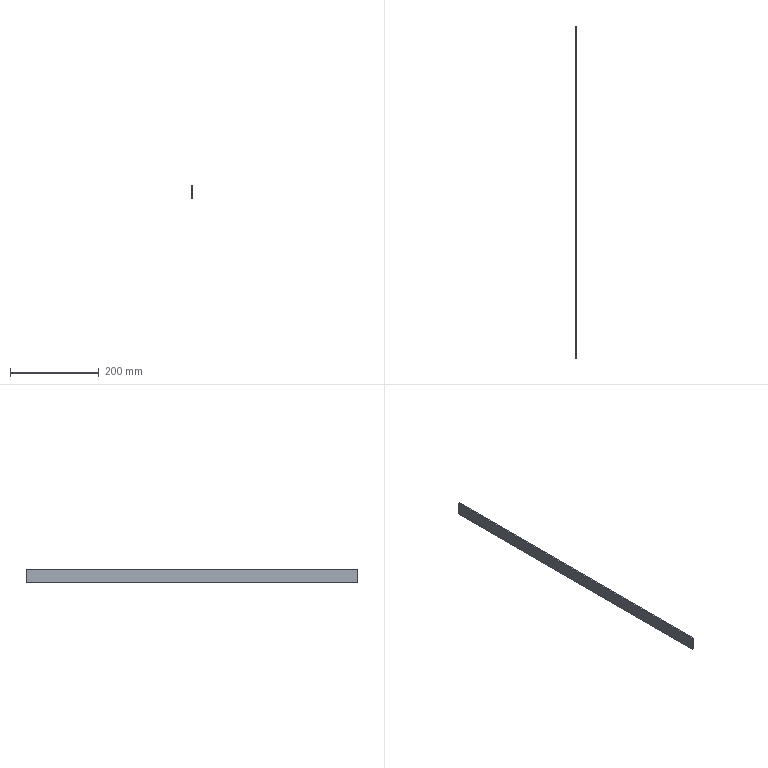Part | SolidWorks | 1 solid | 6 faces | box 3 x 750 x 30 mm | volume 67500 mm3 | plane 6
STEP:
#1=CARTESIAN_POINT('',(0.,375.,15.));
#2=VERTEX_POINT('',#1);
#3=CARTESIAN_POINT('',(0.,-375.,15.));
#4=VERTEX_POINT('',#3);
#5=CARTESIAN_POINT('',(0.,-375.,15.));
#6=DIRECTION('',(0.,-1.,0.));
#7=VECTOR('',#6,1000.);
#8=LINE('',#5,#7);
#9=EDGE_CURVE('',#2,#4,#8,.T.);
#10=ORIENTED_EDGE('',*,*,#9,.F.);
#11=CARTESIAN_POINT('',(-3.,375.,15.));
#12=VERTEX_POINT('',#11);
#13=CARTESIAN_POINT('',(-3.,375.,15.));
#14=DIRECTION('',(1.,0.,0.));
#15=VECTOR('',#14,1000.);
#16=LINE('',#13,#15);
#17=EDGE_CURVE('',#12,#2,#16,.T.);
#18=ORIENTED_EDGE('',*,*,#17,.F.);
#19=CARTESIAN_POINT('',(-3.,-375.,15.));
#20=VERTEX_POINT('',#19);
#21=CARTESIAN_POINT('',(-3.,-375.,15.));
#22=DIRECTION('',(0.,-1.,0.));
#23=VECTOR('',#22,1000.);
#24=LINE('',#21,#23);
#25=EDGE_CURVE('',#12,#20,#24,.T.);
#26=ORIENTED_EDGE('',*,*,#25,.T.);
#27=CARTESIAN_POINT('',(-3.,-375.,15.));
#28=DIRECTION('',(1.,0.,0.));
#29=VECTOR('',#28,1000.);
#30=LINE('',#27,#29);
#31=EDGE_CURVE('',#20,#4,#30,.T.);
#32=ORIENTED_EDGE('',*,*,#31,.T.);
#33=EDGE_LOOP('',(#10,#18,#26,#32));
#34=FACE_OUTER_BOUND('',#33,.T.);
#35=CARTESIAN_POINT('',(-3.,-375.,15.));
#36=DIRECTION('',(0.,0.,1.));
#37=DIRECTION('',(1.,0.,0.));
#38=AXIS2_PLACEMENT_3D('',#35,#36,#37);
#39=PLANE('',#38);
#40=ADVANCED_FACE('',(#34),#39,.T.);
#41=CARTESIAN_POINT('',(0.,375.,-15.));
#42=VERTEX_POINT('',#41);
#43=CARTESIAN_POINT('',(0.,375.,-15.));
#44=DIRECTION('',(0.,0.,1.));
#45=VECTOR('',#44,1000.);
#46=LINE('',#43,#45);
#47=EDGE_CURVE('',#42,#2,#46,.T.);
#48=ORIENTED_EDGE('',*,*,#47,.F.);
#49=CARTESIAN_POINT('',(-3.,375.,-15.));
#50=VERTEX_POINT('',#49);
#51=CARTESIAN_POINT('',(-3.,375.,-15.));
#52=DIRECTION('',(1.,0.,0.));
#53=VECTOR('',#52,1000.);
#54=LINE('',#51,#53);
#55=EDGE_CURVE('',#50,#42,#54,.T.);
#56=ORIENTED_EDGE('',*,*,#55,.F.);
#57=CARTESIAN_POINT('',(-3.,375.,-15.));
#58=DIRECTION('',(0.,0.,1.));
#59=VECTOR('',#58,1000.);
#60=LINE('',#57,#59);
#61=EDGE_CURVE('',#50,#12,#60,.T.);
#62=ORIENTED_EDGE('',*,*,#61,.T.);
#63=ORIENTED_EDGE('',*,*,#17,.T.);
#64=EDGE_LOOP('',(#48,#56,#62,#63));
#65=FACE_OUTER_BOUND('',#64,.T.);
#66=CARTESIAN_POINT('',(-3.,375.,-15.));
#67=DIRECTION('',(0.,1.,0.));
#68=DIRECTION('',(0.,0.,1.));
#69=AXIS2_PLACEMENT_3D('',#66,#67,#68);
#70=PLANE('',#69);
#71=ADVANCED_FACE('',(#65),#70,.T.);
#72=CARTESIAN_POINT('',(0.,-375.,-15.));
#73=VERTEX_POINT('',#72);
#74=CARTESIAN_POINT('',(0.,-375.,-15.));
#75=DIRECTION('',(0.,1.,0.));
#76=VECTOR('',#75,1000.);
#77=LINE('',#74,#76);
#78=EDGE_CURVE('',#73,#42,#77,.T.);
#79=ORIENTED_EDGE('',*,*,#78,.F.);
#80=CARTESIAN_POINT('',(-3.,-375.,-15.));
#81=VERTEX_POINT('',#80);
#82=CARTESIAN_POINT('',(-3.,-375.,-15.));
#83=DIRECTION('',(1.,0.,0.));
#84=VECTOR('',#83,1000.);
#85=LINE('',#82,#84);
#86=EDGE_CURVE('',#81,#73,#85,.T.);
#87=ORIENTED_EDGE('',*,*,#86,.F.);
#88=CARTESIAN_POINT('',(-3.,-375.,-15.));
#89=DIRECTION('',(0.,1.,0.));
#90=VECTOR('',#89,1000.);
#91=LINE('',#88,#90);
#92=EDGE_CURVE('',#81,#50,#91,.T.);
#93=ORIENTED_EDGE('',*,*,#92,.T.);
#94=ORIENTED_EDGE('',*,*,#55,.T.);
#95=EDGE_LOOP('',(#79,#87,#93,#94));
#96=FACE_OUTER_BOUND('',#95,.T.);
#97=CARTESIAN_POINT('',(-3.,-375.,-15.));
#98=DIRECTION('',(0.,0.,-1.));
#99=DIRECTION('',(-1.,0.,0.));
#100=AXIS2_PLACEMENT_3D('',#97,#98,#99);
#101=PLANE('',#100);
#102=ADVANCED_FACE('',(#96),#101,.T.);
#103=CARTESIAN_POINT('',(0.,-375.,-15.));
#104=DIRECTION('',(0.,0.,-1.));
#105=VECTOR('',#104,1000.);
#106=LINE('',#103,#105);
#107=EDGE_CURVE('',#4,#73,#106,.T.);
#108=ORIENTED_EDGE('',*,*,#107,.F.);
#109=ORIENTED_EDGE('',*,*,#31,.F.);
#110=CARTESIAN_POINT('',(-3.,-375.,-15.));
#111=DIRECTION('',(0.,0.,-1.));
#112=VECTOR('',#111,1000.);
#113=LINE('',#110,#112);
#114=EDGE_CURVE('',#20,#81,#113,.T.);
#115=ORIENTED_EDGE('',*,*,#114,.T.);
#116=ORIENTED_EDGE('',*,*,#86,.T.);
#117=EDGE_LOOP('',(#108,#109,#115,#116));
#118=FACE_OUTER_BOUND('',#117,.T.);
#119=CARTESIAN_POINT('',(-3.,-375.,-15.));
#120=DIRECTION('',(0.,-1.,0.));
#121=DIRECTION('',(0.,0.,-1.));
#122=AXIS2_PLACEMENT_3D('',#119,#120,#121);
#123=PLANE('',#122);
#124=ADVANCED_FACE('',(#118),#123,.T.);
#125=ORIENTED_EDGE('',*,*,#25,.F.);
#126=ORIENTED_EDGE('',*,*,#61,.F.);
#127=ORIENTED_EDGE('',*,*,#92,.F.);
#128=ORIENTED_EDGE('',*,*,#114,.F.);
#129=EDGE_LOOP('',(#125,#126,#127,#128));
#130=FACE_OUTER_BOUND('',#129,.T.);
#131=CARTESIAN_POINT('',(-3.,0.,0.));
#132=DIRECTION('',(1.,0.,0.));
#133=DIRECTION('',(0.,0.,-1.));
#134=AXIS2_PLACEMENT_3D('',#131,#132,#133);
#135=PLANE('',#134);
#136=ADVANCED_FACE('',(#130),#135,.F.);
#137=ORIENTED_EDGE('',*,*,#9,.T.);
#138=ORIENTED_EDGE('',*,*,#107,.T.);
#139=ORIENTED_EDGE('',*,*,#78,.T.);
#140=ORIENTED_EDGE('',*,*,#47,.T.);
#141=EDGE_LOOP('',(#137,#138,#139,#140));
#142=FACE_OUTER_BOUND('',#141,.T.);
#143=CARTESIAN_POINT('',(0.,0.,0.));
#144=DIRECTION('',(1.,0.,0.));
#145=DIRECTION('',(0.,0.,-1.));
#146=AXIS2_PLACEMENT_3D('',#143,#144,#145);
#147=PLANE('',#146);
#148=ADVANCED_FACE('',(#142),#147,.T.);
#149=CLOSED_SHELL('',(#40,#71,#102,#124,#136,#148));
#150=MANIFOLD_SOLID_BREP('',#149);
#151=CARTESIAN_POINT('',(0.,0.,0.));
#152=DIRECTION('',(0.,0.,1.));
#153=DIRECTION('',(1.,0.,0.));
#154=AXIS2_PLACEMENT_3D('',#151,#152,#153);
#155=(LENGTH_UNIT()NAMED_UNIT(*)SI_UNIT(.MILLI.,.METRE.));
#156=UNCERTAINTY_MEASURE_WITH_UNIT(LENGTH_MEASURE(0.00001),#155,'','');
#157=(NAMED_UNIT(*)PLANE_ANGLE_UNIT()SI_UNIT($,.RADIAN.));
#158=(NAMED_UNIT(*)SI_UNIT($,.STERADIAN.)SOLID_ANGLE_UNIT());
#159=(GEOMETRIC_REPRESENTATION_CONTEXT(3)GLOBAL_UNCERTAINTY_ASSIGNED_CONTEXT((#156))GLOBAL_UNIT_ASSIGNED_CONTEXT((#155,#157,#158))REPRESENTATION_CONTEXT('',''));
#160=ADVANCED_BREP_SHAPE_REPRESENTATION('',(#150,#154),#159);